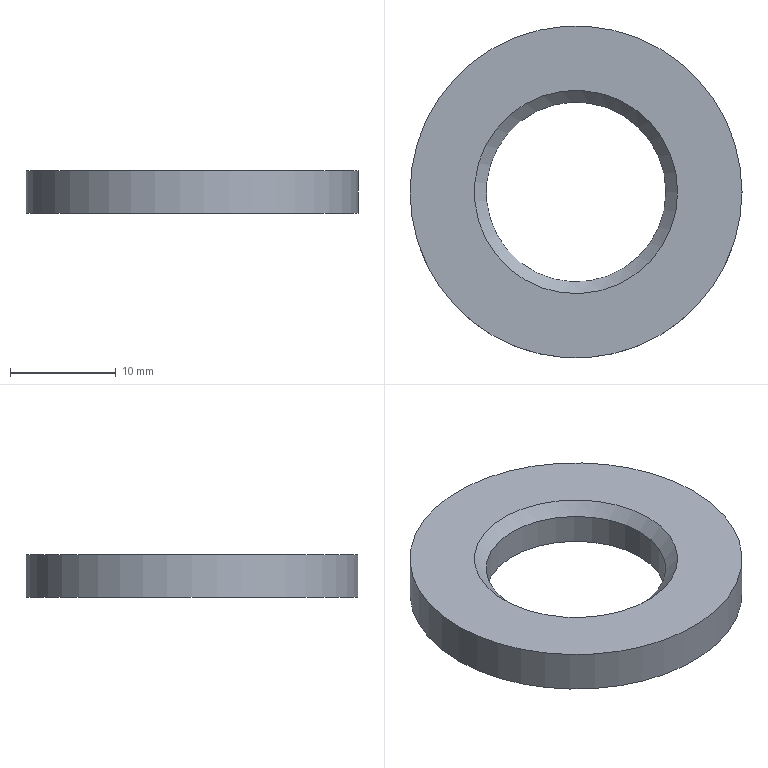Part | STEP file | Washer for steel structures 16 GBT1230-2006_16 | 1 solid | 5 faces | box 31.4 x 31.4 x 4 mm | volume 2155 mm3 | plane 2 | cylinder 2 | cone 1 | commonest cylinder face diameters 17 x1 31.4 x1
STEP:
#1=CARTESIAN_POINT('',(0.,0.,0.));
#2=DIRECTION('',(0.,0.,1.));
#3=DIRECTION('',(1.,0.,0.));
#4=AXIS2_PLACEMENT_3D('',#1,#2,#3);
#5=CARTESIAN_POINT('',(9.615,0.,4.));
#6=VERTEX_POINT('',#5);
#7=CARTESIAN_POINT('',(0.,0.,4.));
#8=DIRECTION('',(0.,0.,1.));
#9=DIRECTION('',(1.,0.,0.));
#10=AXIS2_PLACEMENT_3D('',#7,#8,#9);
#11=CIRCLE('',#10,9.615);
#12=CARTESIAN_POINT('',(0.,0.,4.));
#13=DIRECTION('',(0.,0.,1.));
#14=DIRECTION('',(1.,0.,0.));
#15=AXIS2_PLACEMENT_3D('',#12,#13,#14);
#16=PLANE('',#15);
#17=CARTESIAN_POINT('',(0.,0.));
#18=DIRECTION('',(1.,0.));
#19=AXIS2_PLACEMENT_2D('',#17,#18);
#20=CIRCLE('',#19,9.615);
#21=(GEOMETRIC_REPRESENTATION_CONTEXT(2)PARAMETRIC_REPRESENTATION_CONTEXT()REPRESENTATION_CONTEXT('',''));
#22=DEFINITIONAL_REPRESENTATION('',(#20),#21);
#23=PCURVE('',#16,#22);
#24=CARTESIAN_POINT('',(0.,0.,4.));
#25=DIRECTION('',(0.,0.,1.));
#26=DIRECTION('',(1.,0.,0.));
#27=AXIS2_PLACEMENT_3D('',#24,#25,#26);
#28=CONICAL_SURFACE('',#27,9.615,0.7854);
#29=CARTESIAN_POINT('',(0.,0.));
#30=DIRECTION('',(1.,0.));
#31=VECTOR('',#30,1.);
#32=LINE('',#29,#31);
#33=(GEOMETRIC_REPRESENTATION_CONTEXT(2)PARAMETRIC_REPRESENTATION_CONTEXT()REPRESENTATION_CONTEXT('',''));
#34=DEFINITIONAL_REPRESENTATION('',(#32),#33);
#35=PCURVE('',#28,#34);
#36=SURFACE_CURVE('',#11,(#23,#35),.PCURVE_S1.);
#37=EDGE_CURVE('',#6,#6,#36,.T.);
#38=ORIENTED_EDGE('',*,*,#37,.F.);
#39=EDGE_LOOP('',(#38));
#40=FACE_BOUND('',#39,.T.);
#41=CARTESIAN_POINT('',(15.7,0.,4.));
#42=VERTEX_POINT('',#41);
#43=CARTESIAN_POINT('',(0.,0.,4.));
#44=DIRECTION('',(0.,0.,1.));
#45=DIRECTION('',(1.,0.,0.));
#46=AXIS2_PLACEMENT_3D('',#43,#44,#45);
#47=CIRCLE('',#46,15.7);
#48=CARTESIAN_POINT('',(0.,0.));
#49=DIRECTION('',(1.,0.));
#50=AXIS2_PLACEMENT_2D('',#48,#49);
#51=CIRCLE('',#50,15.7);
#52=(GEOMETRIC_REPRESENTATION_CONTEXT(2)PARAMETRIC_REPRESENTATION_CONTEXT()REPRESENTATION_CONTEXT('',''));
#53=DEFINITIONAL_REPRESENTATION('',(#51),#52);
#54=PCURVE('',#16,#53);
#55=CARTESIAN_POINT('',(0.,0.,4.));
#56=DIRECTION('',(0.,0.,-1.));
#57=DIRECTION('',(-1.,0.,0.));
#58=AXIS2_PLACEMENT_3D('',#55,#56,#57);
#59=CYLINDRICAL_SURFACE('',#58,15.7);
#60=CARTESIAN_POINT('',(9.425,0.));
#61=DIRECTION('',(-1.,0.));
#62=VECTOR('',#61,1.);
#63=LINE('',#60,#62);
#64=(GEOMETRIC_REPRESENTATION_CONTEXT(2)PARAMETRIC_REPRESENTATION_CONTEXT()REPRESENTATION_CONTEXT('',''));
#65=DEFINITIONAL_REPRESENTATION('',(#63),#64);
#66=PCURVE('',#59,#65);
#67=SURFACE_CURVE('',#47,(#54,#66),.PCURVE_S1.);
#68=EDGE_CURVE('',#42,#42,#67,.T.);
#69=ORIENTED_EDGE('',*,*,#68,.T.);
#70=EDGE_LOOP('',(#69));
#71=FACE_BOUND('',#70,.T.);
#72=ADVANCED_FACE('',(#40,#71),#16,.T.);
#73=CARTESIAN_POINT('',(15.7,0.,0.));
#74=VERTEX_POINT('',#73);
#75=CARTESIAN_POINT('',(0.,0.,0.));
#76=DIRECTION('',(0.,0.,1.));
#77=DIRECTION('',(1.,0.,0.));
#78=AXIS2_PLACEMENT_3D('',#75,#76,#77);
#79=CIRCLE('',#78,15.7);
#80=CARTESIAN_POINT('',(0.,0.,0.));
#81=DIRECTION('',(0.,0.,1.));
#82=DIRECTION('',(1.,0.,0.));
#83=AXIS2_PLACEMENT_3D('',#80,#81,#82);
#84=PLANE('',#83);
#85=CARTESIAN_POINT('',(0.,0.));
#86=DIRECTION('',(1.,0.));
#87=AXIS2_PLACEMENT_2D('',#85,#86);
#88=CIRCLE('',#87,15.7);
#89=(GEOMETRIC_REPRESENTATION_CONTEXT(2)PARAMETRIC_REPRESENTATION_CONTEXT()REPRESENTATION_CONTEXT('',''));
#90=DEFINITIONAL_REPRESENTATION('',(#88),#89);
#91=PCURVE('',#84,#90);
#92=CARTESIAN_POINT('',(9.425,4.));
#93=DIRECTION('',(-1.,0.));
#94=VECTOR('',#93,1.);
#95=LINE('',#92,#94);
#96=(GEOMETRIC_REPRESENTATION_CONTEXT(2)PARAMETRIC_REPRESENTATION_CONTEXT()REPRESENTATION_CONTEXT('',''));
#97=DEFINITIONAL_REPRESENTATION('',(#95),#96);
#98=PCURVE('',#59,#97);
#99=SURFACE_CURVE('',#79,(#91,#98),.PCURVE_S1.);
#100=EDGE_CURVE('',#74,#74,#99,.T.);
#101=ORIENTED_EDGE('',*,*,#100,.F.);
#102=EDGE_LOOP('',(#101));
#103=FACE_BOUND('',#102,.T.);
#104=CARTESIAN_POINT('',(8.5,0.,0.));
#105=VERTEX_POINT('',#104);
#106=CARTESIAN_POINT('',(0.,0.,0.));
#107=DIRECTION('',(0.,0.,1.));
#108=DIRECTION('',(1.,0.,0.));
#109=AXIS2_PLACEMENT_3D('',#106,#107,#108);
#110=CIRCLE('',#109,8.5);
#111=CARTESIAN_POINT('',(0.,0.));
#112=DIRECTION('',(1.,0.));
#113=AXIS2_PLACEMENT_2D('',#111,#112);
#114=CIRCLE('',#113,8.5);
#115=(GEOMETRIC_REPRESENTATION_CONTEXT(2)PARAMETRIC_REPRESENTATION_CONTEXT()REPRESENTATION_CONTEXT('',''));
#116=DEFINITIONAL_REPRESENTATION('',(#114),#115);
#117=PCURVE('',#84,#116);
#118=CARTESIAN_POINT('',(0.,0.,4.));
#119=DIRECTION('',(0.,0.,-1.));
#120=DIRECTION('',(-1.,0.,0.));
#121=AXIS2_PLACEMENT_3D('',#118,#119,#120);
#122=CYLINDRICAL_SURFACE('',#121,8.5);
#123=CARTESIAN_POINT('',(9.425,4.));
#124=DIRECTION('',(-1.,0.));
#125=VECTOR('',#124,1.);
#126=LINE('',#123,#125);
#127=(GEOMETRIC_REPRESENTATION_CONTEXT(2)PARAMETRIC_REPRESENTATION_CONTEXT()REPRESENTATION_CONTEXT('',''));
#128=DEFINITIONAL_REPRESENTATION('',(#126),#127);
#129=PCURVE('',#122,#128);
#130=SURFACE_CURVE('',#110,(#117,#129),.PCURVE_S1.);
#131=EDGE_CURVE('',#105,#105,#130,.T.);
#132=ORIENTED_EDGE('',*,*,#131,.T.);
#133=EDGE_LOOP('',(#132));
#134=FACE_BOUND('',#133,.T.);
#135=ADVANCED_FACE('',(#103,#134),#84,.F.);
#136=ORIENTED_EDGE('',*,*,#68,.F.);
#137=CARTESIAN_POINT('',(15.7,0.,4.));
#138=CARTESIAN_POINT('',(15.7,0.,0.));
#139=B_SPLINE_CURVE_WITH_KNOTS('',1,(#137,#138),.UNSPECIFIED.,.F.,.F.,(2,2),(0.,4.),.PIECEWISE_BEZIER_KNOTS.);
#140=CARTESIAN_POINT('',(9.425,0.));
#141=DIRECTION('',(0.,1.));
#142=VECTOR('',#141,1.);
#143=LINE('',#140,#142);
#144=(GEOMETRIC_REPRESENTATION_CONTEXT(2)PARAMETRIC_REPRESENTATION_CONTEXT()REPRESENTATION_CONTEXT('',''));
#145=DEFINITIONAL_REPRESENTATION('',(#143),#144);
#146=PCURVE('',#59,#145);
#147=CARTESIAN_POINT('',(3.142,0.));
#148=DIRECTION('',(0.,1.));
#149=VECTOR('',#148,1.);
#150=LINE('',#147,#149);
#151=(GEOMETRIC_REPRESENTATION_CONTEXT(2)PARAMETRIC_REPRESENTATION_CONTEXT()REPRESENTATION_CONTEXT('',''));
#152=DEFINITIONAL_REPRESENTATION('',(#150),#151);
#153=PCURVE('',#59,#152);
#154=SEAM_CURVE('',#139,(#146,#153),.PCURVE_S1.);
#155=EDGE_CURVE('',#42,#74,#154,.T.);
#156=ORIENTED_EDGE('',*,*,#155,.T.);
#157=ORIENTED_EDGE('',*,*,#100,.T.);
#158=ORIENTED_EDGE('',*,*,#155,.F.);
#159=EDGE_LOOP('',(#136,#156,#157,#158));
#160=FACE_BOUND('',#159,.T.);
#161=ADVANCED_FACE('',(#160),#59,.T.);
#162=CARTESIAN_POINT('',(8.5,0.,2.885));
#163=VERTEX_POINT('',#162);
#164=CARTESIAN_POINT('',(0.,0.,2.885));
#165=DIRECTION('',(0.,0.,-1.));
#166=DIRECTION('',(1.,0.,0.));
#167=AXIS2_PLACEMENT_3D('',#164,#165,#166);
#168=CIRCLE('',#167,8.5);
#169=CARTESIAN_POINT('',(3.142,1.115));
#170=DIRECTION('',(1.,0.));
#171=VECTOR('',#170,1.);
#172=LINE('',#169,#171);
#173=(GEOMETRIC_REPRESENTATION_CONTEXT(2)PARAMETRIC_REPRESENTATION_CONTEXT()REPRESENTATION_CONTEXT('',''));
#174=DEFINITIONAL_REPRESENTATION('',(#172),#173);
#175=PCURVE('',#122,#174);
#176=CARTESIAN_POINT('',(6.283,-1.115));
#177=DIRECTION('',(-1.,0.));
#178=VECTOR('',#177,1.);
#179=LINE('',#176,#178);
#180=(GEOMETRIC_REPRESENTATION_CONTEXT(2)PARAMETRIC_REPRESENTATION_CONTEXT()REPRESENTATION_CONTEXT('',''));
#181=DEFINITIONAL_REPRESENTATION('',(#179),#180);
#182=PCURVE('',#28,#181);
#183=SURFACE_CURVE('',#168,(#175,#182),.PCURVE_S1.);
#184=EDGE_CURVE('',#163,#163,#183,.T.);
#185=ORIENTED_EDGE('',*,*,#184,.T.);
#186=CARTESIAN_POINT('',(8.5,0.,2.885));
#187=CARTESIAN_POINT('',(8.5,0.,0.));
#188=B_SPLINE_CURVE_WITH_KNOTS('',1,(#186,#187),.UNSPECIFIED.,.F.,.F.,(2,2),(1.115,4.),.PIECEWISE_BEZIER_KNOTS.);
#189=CARTESIAN_POINT('',(9.425,0.));
#190=DIRECTION('',(0.,1.));
#191=VECTOR('',#190,1.);
#192=LINE('',#189,#191);
#193=(GEOMETRIC_REPRESENTATION_CONTEXT(2)PARAMETRIC_REPRESENTATION_CONTEXT()REPRESENTATION_CONTEXT('',''));
#194=DEFINITIONAL_REPRESENTATION('',(#192),#193);
#195=PCURVE('',#122,#194);
#196=CARTESIAN_POINT('',(3.142,0.));
#197=DIRECTION('',(0.,1.));
#198=VECTOR('',#197,1.);
#199=LINE('',#196,#198);
#200=(GEOMETRIC_REPRESENTATION_CONTEXT(2)PARAMETRIC_REPRESENTATION_CONTEXT()REPRESENTATION_CONTEXT('',''));
#201=DEFINITIONAL_REPRESENTATION('',(#199),#200);
#202=PCURVE('',#122,#201);
#203=SEAM_CURVE('',#188,(#195,#202),.PCURVE_S1.);
#204=EDGE_CURVE('',#163,#105,#203,.T.);
#205=ORIENTED_EDGE('',*,*,#204,.T.);
#206=ORIENTED_EDGE('',*,*,#131,.T.);
#207=ORIENTED_EDGE('',*,*,#204,.F.);
#208=EDGE_LOOP('',(#185,#205,#206,#207));
#209=FACE_BOUND('',#208,.F.);
#210=ADVANCED_FACE('',(#209),#122,.F.);
#211=ORIENTED_EDGE('',*,*,#184,.F.);
#212=CARTESIAN_POINT('',(8.5,0.,2.885));
#213=CARTESIAN_POINT('',(9.615,0.,4.));
#214=B_SPLINE_CURVE_WITH_KNOTS('',1,(#212,#213),.UNSPECIFIED.,.F.,.F.,(2,2),(-1.577,0.),.PIECEWISE_BEZIER_KNOTS.);
#215=CARTESIAN_POINT('',(6.283,0.));
#216=DIRECTION('',(0.,1.));
#217=VECTOR('',#216,1.);
#218=LINE('',#215,#217);
#219=(GEOMETRIC_REPRESENTATION_CONTEXT(2)PARAMETRIC_REPRESENTATION_CONTEXT()REPRESENTATION_CONTEXT('',''));
#220=DEFINITIONAL_REPRESENTATION('',(#218),#219);
#221=PCURVE('',#28,#220);
#222=CARTESIAN_POINT('',(0.,0.));
#223=DIRECTION('',(0.,1.));
#224=VECTOR('',#223,1.);
#225=LINE('',#222,#224);
#226=(GEOMETRIC_REPRESENTATION_CONTEXT(2)PARAMETRIC_REPRESENTATION_CONTEXT()REPRESENTATION_CONTEXT('',''));
#227=DEFINITIONAL_REPRESENTATION('',(#225),#226);
#228=PCURVE('',#28,#227);
#229=SEAM_CURVE('',#214,(#221,#228),.PCURVE_S1.);
#230=EDGE_CURVE('',#163,#6,#229,.T.);
#231=ORIENTED_EDGE('',*,*,#230,.T.);
#232=ORIENTED_EDGE('',*,*,#37,.F.);
#233=ORIENTED_EDGE('',*,*,#230,.F.);
#234=EDGE_LOOP('',(#211,#231,#232,#233));
#235=FACE_BOUND('',#234,.F.);
#236=ADVANCED_FACE('',(#235),#28,.F.);
#237=CLOSED_SHELL('',(#72,#135,#161,#210,#236));
#238=MANIFOLD_SOLID_BREP('',#237);
#239=(LENGTH_UNIT()NAMED_UNIT(*)SI_UNIT(.MILLI.,.METRE.));
#240=UNCERTAINTY_MEASURE_WITH_UNIT(LENGTH_MEASURE(0.00001),#239,'','');
#241=(NAMED_UNIT(*)PLANE_ANGLE_UNIT()SI_UNIT($,.RADIAN.));
#242=(NAMED_UNIT(*)SI_UNIT($,.STERADIAN.)SOLID_ANGLE_UNIT());
#243=(GEOMETRIC_REPRESENTATION_CONTEXT(3)GLOBAL_UNCERTAINTY_ASSIGNED_CONTEXT((#240))GLOBAL_UNIT_ASSIGNED_CONTEXT((#239,#241,#242))REPRESENTATION_CONTEXT('',''));
#244=ADVANCED_BREP_SHAPE_REPRESENTATION('',(#4,#238),#243);